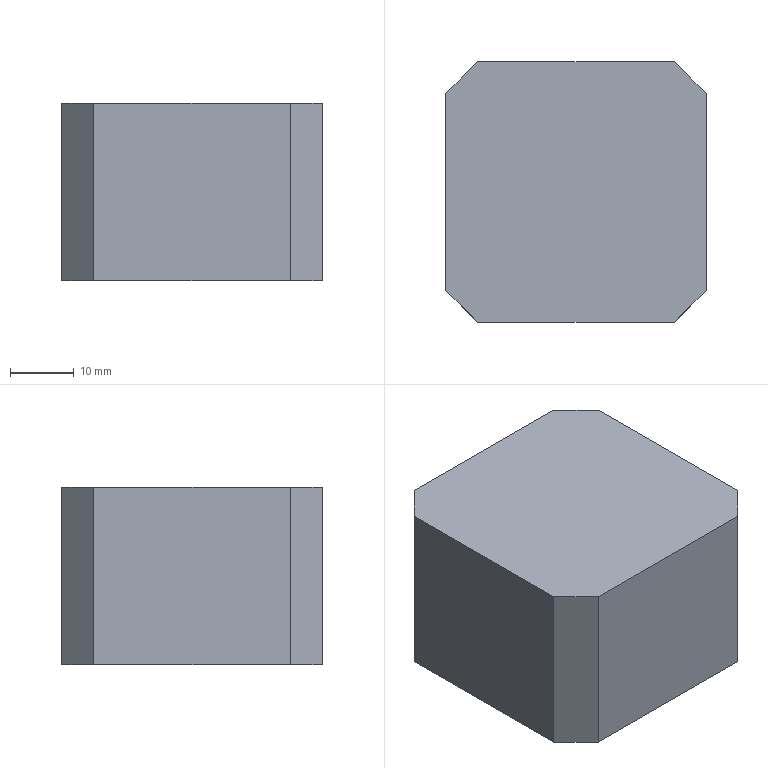Part | SolidWorks | features BaseBody 1 | 1 solid | 10 faces | box 41 x 41 x 28 mm | volume 45668 mm3 | plane 10
STEP:
#1=CARTESIAN_POINT('',(10.948,-7.87,28.));
#2=VERTEX_POINT('',#1);
#3=CARTESIAN_POINT('',(10.948,23.13,28.));
#4=VERTEX_POINT('',#3);
#5=CARTESIAN_POINT('',(10.948,7.63,28.));
#6=DIRECTION('',(0.,1.,0.));
#7=VECTOR('',#6,1000.);
#8=LINE('',#5,#7);
#9=EDGE_CURVE('',#2,#4,#8,.T.);
#10=ORIENTED_EDGE('',*,*,#9,.T.);
#11=CARTESIAN_POINT('',(5.948,28.13,28.));
#12=VERTEX_POINT('',#11);
#13=CARTESIAN_POINT('',(10.948,23.13,28.));
#14=DIRECTION('',(-0.7071,0.7071,0.));
#15=VECTOR('',#14,1000.);
#16=LINE('',#13,#15);
#17=EDGE_CURVE('',#4,#12,#16,.T.);
#18=ORIENTED_EDGE('',*,*,#17,.T.);
#19=CARTESIAN_POINT('',(-25.052,28.13,28.));
#20=VERTEX_POINT('',#19);
#21=CARTESIAN_POINT('',(-9.552,28.13,28.));
#22=DIRECTION('',(-1.,0.,0.));
#23=VECTOR('',#22,1000.);
#24=LINE('',#21,#23);
#25=EDGE_CURVE('',#12,#20,#24,.T.);
#26=ORIENTED_EDGE('',*,*,#25,.T.);
#27=CARTESIAN_POINT('',(-30.052,23.13,28.));
#28=VERTEX_POINT('',#27);
#29=CARTESIAN_POINT('',(-25.052,28.13,28.));
#30=DIRECTION('',(-0.7071,-0.7071,0.));
#31=VECTOR('',#30,1000.);
#32=LINE('',#29,#31);
#33=EDGE_CURVE('',#20,#28,#32,.T.);
#34=ORIENTED_EDGE('',*,*,#33,.T.);
#35=CARTESIAN_POINT('',(-30.052,-7.87,28.));
#36=VERTEX_POINT('',#35);
#37=CARTESIAN_POINT('',(-30.052,7.63,28.));
#38=DIRECTION('',(0.,-1.,0.));
#39=VECTOR('',#38,1000.);
#40=LINE('',#37,#39);
#41=EDGE_CURVE('',#28,#36,#40,.T.);
#42=ORIENTED_EDGE('',*,*,#41,.T.);
#43=CARTESIAN_POINT('',(-25.052,-12.87,28.));
#44=VERTEX_POINT('',#43);
#45=CARTESIAN_POINT('',(-30.052,-7.87,28.));
#46=DIRECTION('',(0.7071,-0.7071,0.));
#47=VECTOR('',#46,1000.);
#48=LINE('',#45,#47);
#49=EDGE_CURVE('',#36,#44,#48,.T.);
#50=ORIENTED_EDGE('',*,*,#49,.T.);
#51=CARTESIAN_POINT('',(5.948,-12.87,28.));
#52=VERTEX_POINT('',#51);
#53=CARTESIAN_POINT('',(-9.552,-12.87,28.));
#54=DIRECTION('',(1.,0.,0.));
#55=VECTOR('',#54,1000.);
#56=LINE('',#53,#55);
#57=EDGE_CURVE('',#44,#52,#56,.T.);
#58=ORIENTED_EDGE('',*,*,#57,.T.);
#59=CARTESIAN_POINT('',(5.948,-12.87,28.));
#60=DIRECTION('',(0.7071,0.7071,0.));
#61=VECTOR('',#60,1000.);
#62=LINE('',#59,#61);
#63=EDGE_CURVE('',#52,#2,#62,.T.);
#64=ORIENTED_EDGE('',*,*,#63,.T.);
#65=EDGE_LOOP('',(#10,#18,#26,#34,#42,#50,#58,#64));
#66=FACE_OUTER_BOUND('',#65,.T.);
#67=CARTESIAN_POINT('',(-9.552,7.63,28.));
#68=DIRECTION('',(0.,0.,1.));
#69=DIRECTION('',(1.,0.,0.));
#70=AXIS2_PLACEMENT_3D('',#67,#68,#69);
#71=PLANE('',#70);
#72=ADVANCED_FACE('',(#66),#71,.T.);
#73=CARTESIAN_POINT('',(10.948,23.13,0.));
#74=VERTEX_POINT('',#73);
#75=CARTESIAN_POINT('',(5.948,28.13,0.));
#76=VERTEX_POINT('',#75);
#77=CARTESIAN_POINT('',(5.948,28.13,0.));
#78=DIRECTION('',(-0.7071,0.7071,0.));
#79=VECTOR('',#78,1000.);
#80=LINE('',#77,#79);
#81=EDGE_CURVE('',#74,#76,#80,.T.);
#82=ORIENTED_EDGE('',*,*,#81,.T.);
#83=CARTESIAN_POINT('',(5.948,28.13,0.));
#84=DIRECTION('',(0.,0.,1.));
#85=VECTOR('',#84,1000.);
#86=LINE('',#83,#85);
#87=EDGE_CURVE('',#76,#12,#86,.T.);
#88=ORIENTED_EDGE('',*,*,#87,.T.);
#89=ORIENTED_EDGE('',*,*,#17,.F.);
#90=CARTESIAN_POINT('',(10.948,23.13,0.));
#91=DIRECTION('',(0.,0.,-1.));
#92=VECTOR('',#91,1000.);
#93=LINE('',#90,#92);
#94=EDGE_CURVE('',#4,#74,#93,.T.);
#95=ORIENTED_EDGE('',*,*,#94,.T.);
#96=EDGE_LOOP('',(#82,#88,#89,#95));
#97=FACE_OUTER_BOUND('',#96,.T.);
#98=CARTESIAN_POINT('',(5.948,28.13,0.));
#99=DIRECTION('',(0.7071,0.7071,0.));
#100=DIRECTION('',(-0.7071,0.7071,0.));
#101=AXIS2_PLACEMENT_3D('',#98,#99,#100);
#102=PLANE('',#101);
#103=ADVANCED_FACE('',(#97),#102,.T.);
#104=CARTESIAN_POINT('',(10.948,-7.87,0.));
#105=VERTEX_POINT('',#104);
#106=CARTESIAN_POINT('',(10.948,23.13,0.));
#107=DIRECTION('',(0.,1.,0.));
#108=VECTOR('',#107,1000.);
#109=LINE('',#106,#108);
#110=EDGE_CURVE('',#105,#74,#109,.T.);
#111=ORIENTED_EDGE('',*,*,#110,.T.);
#112=ORIENTED_EDGE('',*,*,#94,.F.);
#113=ORIENTED_EDGE('',*,*,#9,.F.);
#114=CARTESIAN_POINT('',(10.948,-7.87,0.));
#115=DIRECTION('',(0.,0.,-1.));
#116=VECTOR('',#115,1000.);
#117=LINE('',#114,#116);
#118=EDGE_CURVE('',#2,#105,#117,.T.);
#119=ORIENTED_EDGE('',*,*,#118,.T.);
#120=EDGE_LOOP('',(#111,#112,#113,#119));
#121=FACE_OUTER_BOUND('',#120,.T.);
#122=CARTESIAN_POINT('',(10.948,23.13,0.));
#123=DIRECTION('',(1.,0.,0.));
#124=DIRECTION('',(0.,0.,-1.));
#125=AXIS2_PLACEMENT_3D('',#122,#123,#124);
#126=PLANE('',#125);
#127=ADVANCED_FACE('',(#121),#126,.T.);
#128=CARTESIAN_POINT('',(5.948,-12.87,0.));
#129=VERTEX_POINT('',#128);
#130=CARTESIAN_POINT('',(10.948,-7.87,0.));
#131=DIRECTION('',(0.7071,0.7071,0.));
#132=VECTOR('',#131,1000.);
#133=LINE('',#130,#132);
#134=EDGE_CURVE('',#129,#105,#133,.T.);
#135=ORIENTED_EDGE('',*,*,#134,.T.);
#136=ORIENTED_EDGE('',*,*,#118,.F.);
#137=ORIENTED_EDGE('',*,*,#63,.F.);
#138=CARTESIAN_POINT('',(5.948,-12.87,0.));
#139=DIRECTION('',(0.,0.,-1.));
#140=VECTOR('',#139,1000.);
#141=LINE('',#138,#140);
#142=EDGE_CURVE('',#52,#129,#141,.T.);
#143=ORIENTED_EDGE('',*,*,#142,.T.);
#144=EDGE_LOOP('',(#135,#136,#137,#143));
#145=FACE_OUTER_BOUND('',#144,.T.);
#146=CARTESIAN_POINT('',(10.948,-7.87,0.));
#147=DIRECTION('',(0.7071,-0.7071,0.));
#148=DIRECTION('',(0.7071,0.7071,0.));
#149=AXIS2_PLACEMENT_3D('',#146,#147,#148);
#150=PLANE('',#149);
#151=ADVANCED_FACE('',(#145),#150,.T.);
#152=CARTESIAN_POINT('',(-25.052,-12.87,0.));
#153=VERTEX_POINT('',#152);
#154=CARTESIAN_POINT('',(5.948,-12.87,0.));
#155=DIRECTION('',(1.,0.,0.));
#156=VECTOR('',#155,1000.);
#157=LINE('',#154,#156);
#158=EDGE_CURVE('',#153,#129,#157,.T.);
#159=ORIENTED_EDGE('',*,*,#158,.T.);
#160=ORIENTED_EDGE('',*,*,#142,.F.);
#161=ORIENTED_EDGE('',*,*,#57,.F.);
#162=CARTESIAN_POINT('',(-25.052,-12.87,0.));
#163=DIRECTION('',(0.,0.,-1.));
#164=VECTOR('',#163,1000.);
#165=LINE('',#162,#164);
#166=EDGE_CURVE('',#44,#153,#165,.T.);
#167=ORIENTED_EDGE('',*,*,#166,.T.);
#168=EDGE_LOOP('',(#159,#160,#161,#167));
#169=FACE_OUTER_BOUND('',#168,.T.);
#170=CARTESIAN_POINT('',(5.948,-12.87,0.));
#171=DIRECTION('',(0.,-1.,0.));
#172=DIRECTION('',(0.,0.,-1.));
#173=AXIS2_PLACEMENT_3D('',#170,#171,#172);
#174=PLANE('',#173);
#175=ADVANCED_FACE('',(#169),#174,.T.);
#176=CARTESIAN_POINT('',(-30.052,-7.87,0.));
#177=VERTEX_POINT('',#176);
#178=CARTESIAN_POINT('',(-25.052,-12.87,0.));
#179=DIRECTION('',(0.7071,-0.7071,0.));
#180=VECTOR('',#179,1000.);
#181=LINE('',#178,#180);
#182=EDGE_CURVE('',#177,#153,#181,.T.);
#183=ORIENTED_EDGE('',*,*,#182,.T.);
#184=ORIENTED_EDGE('',*,*,#166,.F.);
#185=ORIENTED_EDGE('',*,*,#49,.F.);
#186=CARTESIAN_POINT('',(-30.052,-7.87,0.));
#187=DIRECTION('',(0.,0.,-1.));
#188=VECTOR('',#187,1000.);
#189=LINE('',#186,#188);
#190=EDGE_CURVE('',#36,#177,#189,.T.);
#191=ORIENTED_EDGE('',*,*,#190,.T.);
#192=EDGE_LOOP('',(#183,#184,#185,#191));
#193=FACE_OUTER_BOUND('',#192,.T.);
#194=CARTESIAN_POINT('',(-25.052,-12.87,0.));
#195=DIRECTION('',(-0.7071,-0.7071,0.));
#196=DIRECTION('',(0.7071,-0.7071,0.));
#197=AXIS2_PLACEMENT_3D('',#194,#195,#196);
#198=PLANE('',#197);
#199=ADVANCED_FACE('',(#193),#198,.T.);
#200=CARTESIAN_POINT('',(-30.052,23.13,0.));
#201=VERTEX_POINT('',#200);
#202=CARTESIAN_POINT('',(-30.052,-7.87,0.));
#203=DIRECTION('',(0.,-1.,0.));
#204=VECTOR('',#203,1000.);
#205=LINE('',#202,#204);
#206=EDGE_CURVE('',#201,#177,#205,.T.);
#207=ORIENTED_EDGE('',*,*,#206,.T.);
#208=ORIENTED_EDGE('',*,*,#190,.F.);
#209=ORIENTED_EDGE('',*,*,#41,.F.);
#210=CARTESIAN_POINT('',(-30.052,23.13,0.));
#211=DIRECTION('',(0.,0.,-1.));
#212=VECTOR('',#211,1000.);
#213=LINE('',#210,#212);
#214=EDGE_CURVE('',#28,#201,#213,.T.);
#215=ORIENTED_EDGE('',*,*,#214,.T.);
#216=EDGE_LOOP('',(#207,#208,#209,#215));
#217=FACE_OUTER_BOUND('',#216,.T.);
#218=CARTESIAN_POINT('',(-30.052,-7.87,0.));
#219=DIRECTION('',(-1.,0.,0.));
#220=DIRECTION('',(0.,0.,1.));
#221=AXIS2_PLACEMENT_3D('',#218,#219,#220);
#222=PLANE('',#221);
#223=ADVANCED_FACE('',(#217),#222,.T.);
#224=CARTESIAN_POINT('',(-25.052,28.13,0.));
#225=VERTEX_POINT('',#224);
#226=CARTESIAN_POINT('',(-30.052,23.13,0.));
#227=DIRECTION('',(-0.7071,-0.7071,0.));
#228=VECTOR('',#227,1000.);
#229=LINE('',#226,#228);
#230=EDGE_CURVE('',#225,#201,#229,.T.);
#231=ORIENTED_EDGE('',*,*,#230,.T.);
#232=ORIENTED_EDGE('',*,*,#214,.F.);
#233=ORIENTED_EDGE('',*,*,#33,.F.);
#234=CARTESIAN_POINT('',(-25.052,28.13,0.));
#235=DIRECTION('',(0.,0.,-1.));
#236=VECTOR('',#235,1000.);
#237=LINE('',#234,#236);
#238=EDGE_CURVE('',#20,#225,#237,.T.);
#239=ORIENTED_EDGE('',*,*,#238,.T.);
#240=EDGE_LOOP('',(#231,#232,#233,#239));
#241=FACE_OUTER_BOUND('',#240,.T.);
#242=CARTESIAN_POINT('',(-30.052,23.13,0.));
#243=DIRECTION('',(-0.7071,0.7071,0.));
#244=DIRECTION('',(-0.7071,-0.7071,0.));
#245=AXIS2_PLACEMENT_3D('',#242,#243,#244);
#246=PLANE('',#245);
#247=ADVANCED_FACE('',(#241),#246,.T.);
#248=CARTESIAN_POINT('',(-25.052,28.13,0.));
#249=DIRECTION('',(-1.,0.,0.));
#250=VECTOR('',#249,1000.);
#251=LINE('',#248,#250);
#252=EDGE_CURVE('',#76,#225,#251,.T.);
#253=ORIENTED_EDGE('',*,*,#252,.T.);
#254=ORIENTED_EDGE('',*,*,#238,.F.);
#255=ORIENTED_EDGE('',*,*,#25,.F.);
#256=ORIENTED_EDGE('',*,*,#87,.F.);
#257=EDGE_LOOP('',(#253,#254,#255,#256));
#258=FACE_OUTER_BOUND('',#257,.T.);
#259=CARTESIAN_POINT('',(-25.052,28.13,0.));
#260=DIRECTION('',(0.,1.,0.));
#261=DIRECTION('',(0.,0.,1.));
#262=AXIS2_PLACEMENT_3D('',#259,#260,#261);
#263=PLANE('',#262);
#264=ADVANCED_FACE('',(#258),#263,.T.);
#265=ORIENTED_EDGE('',*,*,#252,.F.);
#266=ORIENTED_EDGE('',*,*,#81,.F.);
#267=ORIENTED_EDGE('',*,*,#110,.F.);
#268=ORIENTED_EDGE('',*,*,#134,.F.);
#269=ORIENTED_EDGE('',*,*,#158,.F.);
#270=ORIENTED_EDGE('',*,*,#182,.F.);
#271=ORIENTED_EDGE('',*,*,#206,.F.);
#272=ORIENTED_EDGE('',*,*,#230,.F.);
#273=EDGE_LOOP('',(#265,#266,#267,#268,#269,#270,#271,#272));
#274=FACE_OUTER_BOUND('',#273,.T.);
#275=CARTESIAN_POINT('',(-9.552,7.63,0.));
#276=DIRECTION('',(0.,0.,1.));
#277=DIRECTION('',(1.,0.,0.));
#278=AXIS2_PLACEMENT_3D('',#275,#276,#277);
#279=PLANE('',#278);
#280=ADVANCED_FACE('',(#274),#279,.F.);
#281=CLOSED_SHELL('',(#72,#103,#127,#151,#175,#199,#223,#247,#264,#280));
#282=MANIFOLD_SOLID_BREP('',#281);
#283=CARTESIAN_POINT('',(0.,0.,0.));
#284=DIRECTION('',(0.,0.,1.));
#285=DIRECTION('',(1.,0.,0.));
#286=AXIS2_PLACEMENT_3D('',#283,#284,#285);
#287=(LENGTH_UNIT()NAMED_UNIT(*)SI_UNIT(.MILLI.,.METRE.));
#288=UNCERTAINTY_MEASURE_WITH_UNIT(LENGTH_MEASURE(0.00001),#287,'','');
#289=(NAMED_UNIT(*)PLANE_ANGLE_UNIT()SI_UNIT($,.RADIAN.));
#290=(NAMED_UNIT(*)SI_UNIT($,.STERADIAN.)SOLID_ANGLE_UNIT());
#291=(GEOMETRIC_REPRESENTATION_CONTEXT(3)GLOBAL_UNCERTAINTY_ASSIGNED_CONTEXT((#288))GLOBAL_UNIT_ASSIGNED_CONTEXT((#287,#289,#290))REPRESENTATION_CONTEXT('',''));
#292=ADVANCED_BREP_SHAPE_REPRESENTATION('',(#282,#286),#291);